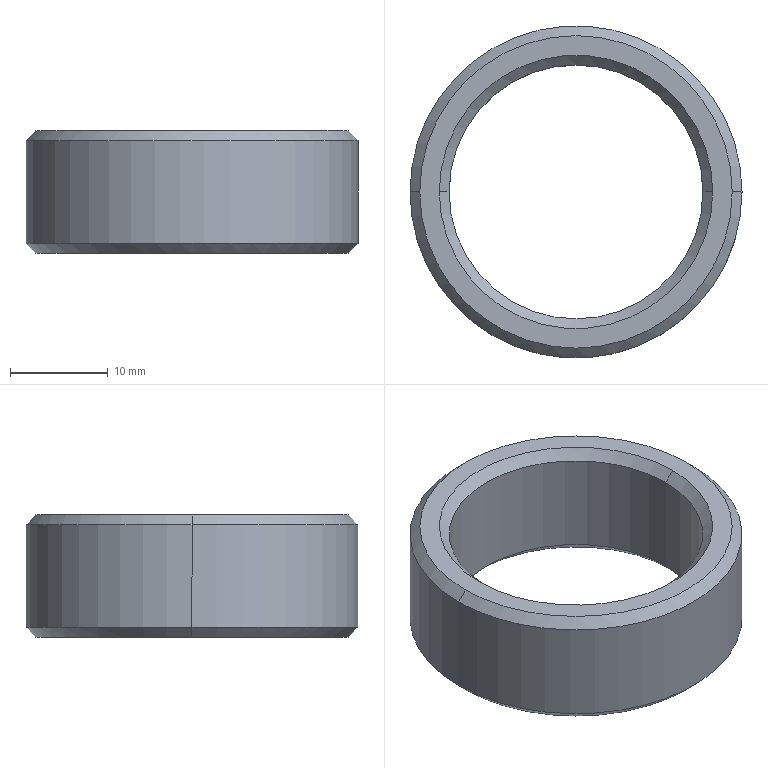Part | STEP file | 1 solid | 14 faces | box 34 x 34 x 12.5 mm | volume 4524 mm3 | cone 8 | cylinder 4 | plane 2 | commonest cylinder face diameters 26 x2 34 x2
STEP:
#1=CARTESIAN_POINT('',(0.,0.,0.));
#2=DIRECTION('',(0.,0.,1.));
#3=DIRECTION('',(1.,0.,0.));
#4=AXIS2_PLACEMENT_3D('',#1,#2,#3);
#5=CARTESIAN_POINT('',(-13.,0.,1.));
#6=VERTEX_POINT('',#5);
#7=CARTESIAN_POINT('',(13.,0.,1.));
#8=VERTEX_POINT('',#7);
#9=CARTESIAN_POINT('',(0.,0.,1.));
#10=DIRECTION('',(0.,0.,-1.));
#11=DIRECTION('',(-1.,0.,0.));
#12=AXIS2_PLACEMENT_3D('',#9,#10,#11);
#13=CIRCLE('',#12,13.);
#14=CARTESIAN_POINT('',(0.,0.,12.5));
#15=DIRECTION('',(0.,0.,-1.));
#16=DIRECTION('',(-1.,0.,0.));
#17=AXIS2_PLACEMENT_3D('',#14,#15,#16);
#18=CYLINDRICAL_SURFACE('',#17,13.);
#19=CARTESIAN_POINT('',(0.,11.5));
#20=DIRECTION('',(1.,0.));
#21=VECTOR('',#20,1.);
#22=LINE('',#19,#21);
#23=(GEOMETRIC_REPRESENTATION_CONTEXT(2)PARAMETRIC_REPRESENTATION_CONTEXT()REPRESENTATION_CONTEXT('',''));
#24=DEFINITIONAL_REPRESENTATION('',(#22),#23);
#25=PCURVE('',#18,#24);
#26=CARTESIAN_POINT('',(0.,0.,0.));
#27=DIRECTION('',(0.,0.,-1.));
#28=DIRECTION('',(-1.,0.,0.));
#29=AXIS2_PLACEMENT_3D('',#26,#27,#28);
#30=CONICAL_SURFACE('',#29,14.,0.7854);
#31=CARTESIAN_POINT('',(0.,-1.));
#32=DIRECTION('',(1.,0.));
#33=VECTOR('',#32,1.);
#34=LINE('',#31,#33);
#35=(GEOMETRIC_REPRESENTATION_CONTEXT(2)PARAMETRIC_REPRESENTATION_CONTEXT()REPRESENTATION_CONTEXT('',''));
#36=DEFINITIONAL_REPRESENTATION('',(#34),#35);
#37=PCURVE('',#30,#36);
#38=SURFACE_CURVE('',#13,(#25,#37),.PCURVE_S1.);
#39=EDGE_CURVE('',#6,#8,#38,.T.);
#40=ORIENTED_EDGE('',*,*,#39,.F.);
#41=CARTESIAN_POINT('',(-13.,0.,11.5));
#42=VERTEX_POINT('',#41);
#43=CARTESIAN_POINT('',(-13.,0.,12.5));
#44=DIRECTION('',(0.,0.,-1.));
#45=VECTOR('',#44,1.);
#46=LINE('',#43,#45);
#47=CARTESIAN_POINT('',(0.,0.));
#48=DIRECTION('',(0.,1.));
#49=VECTOR('',#48,1.);
#50=LINE('',#47,#49);
#51=(GEOMETRIC_REPRESENTATION_CONTEXT(2)PARAMETRIC_REPRESENTATION_CONTEXT()REPRESENTATION_CONTEXT('',''));
#52=DEFINITIONAL_REPRESENTATION('',(#50),#51);
#53=PCURVE('',#18,#52);
#54=CARTESIAN_POINT('',(0.,0.,12.5));
#55=DIRECTION('',(0.,0.,-1.));
#56=DIRECTION('',(-1.,0.,0.));
#57=AXIS2_PLACEMENT_3D('',#54,#55,#56);
#58=CYLINDRICAL_SURFACE('',#57,13.);
#59=CARTESIAN_POINT('',(6.283,0.));
#60=DIRECTION('',(0.,1.));
#61=VECTOR('',#60,1.);
#62=LINE('',#59,#61);
#63=(GEOMETRIC_REPRESENTATION_CONTEXT(2)PARAMETRIC_REPRESENTATION_CONTEXT()REPRESENTATION_CONTEXT('',''));
#64=DEFINITIONAL_REPRESENTATION('',(#62),#63);
#65=PCURVE('',#58,#64);
#66=SURFACE_CURVE('',#46,(#53,#65),.PCURVE_S1.);
#67=EDGE_CURVE('',#42,#6,#66,.T.);
#68=ORIENTED_EDGE('',*,*,#67,.F.);
#69=CARTESIAN_POINT('',(13.,0.,11.5));
#70=VERTEX_POINT('',#69);
#71=CARTESIAN_POINT('',(0.,0.,11.5));
#72=DIRECTION('',(0.,0.,1.));
#73=DIRECTION('',(1.,0.,0.));
#74=AXIS2_PLACEMENT_3D('',#71,#72,#73);
#75=CIRCLE('',#74,13.);
#76=CARTESIAN_POINT('',(3.142,1.));
#77=DIRECTION('',(-1.,0.));
#78=VECTOR('',#77,1.);
#79=LINE('',#76,#78);
#80=(GEOMETRIC_REPRESENTATION_CONTEXT(2)PARAMETRIC_REPRESENTATION_CONTEXT()REPRESENTATION_CONTEXT('',''));
#81=DEFINITIONAL_REPRESENTATION('',(#79),#80);
#82=PCURVE('',#18,#81);
#83=CARTESIAN_POINT('',(0.,0.,12.5));
#84=DIRECTION('',(0.,0.,1.));
#85=DIRECTION('',(1.,0.,0.));
#86=AXIS2_PLACEMENT_3D('',#83,#84,#85);
#87=CONICAL_SURFACE('',#86,14.,0.7854);
#88=CARTESIAN_POINT('',(0.,-1.));
#89=DIRECTION('',(1.,0.));
#90=VECTOR('',#89,1.);
#91=LINE('',#88,#90);
#92=(GEOMETRIC_REPRESENTATION_CONTEXT(2)PARAMETRIC_REPRESENTATION_CONTEXT()REPRESENTATION_CONTEXT('',''));
#93=DEFINITIONAL_REPRESENTATION('',(#91),#92);
#94=PCURVE('',#87,#93);
#95=SURFACE_CURVE('',#75,(#82,#94),.PCURVE_S1.);
#96=EDGE_CURVE('',#70,#42,#95,.T.);
#97=ORIENTED_EDGE('',*,*,#96,.F.);
#98=CARTESIAN_POINT('',(13.,0.,12.5));
#99=DIRECTION('',(0.,0.,-1.));
#100=VECTOR('',#99,1.);
#101=LINE('',#98,#100);
#102=CARTESIAN_POINT('',(3.142,0.));
#103=DIRECTION('',(0.,1.));
#104=VECTOR('',#103,1.);
#105=LINE('',#102,#104);
#106=(GEOMETRIC_REPRESENTATION_CONTEXT(2)PARAMETRIC_REPRESENTATION_CONTEXT()REPRESENTATION_CONTEXT('',''));
#107=DEFINITIONAL_REPRESENTATION('',(#105),#106);
#108=PCURVE('',#18,#107);
#109=CARTESIAN_POINT('',(3.142,0.));
#110=DIRECTION('',(0.,1.));
#111=VECTOR('',#110,1.);
#112=LINE('',#109,#111);
#113=(GEOMETRIC_REPRESENTATION_CONTEXT(2)PARAMETRIC_REPRESENTATION_CONTEXT()REPRESENTATION_CONTEXT('',''));
#114=DEFINITIONAL_REPRESENTATION('',(#112),#113);
#115=PCURVE('',#58,#114);
#116=SURFACE_CURVE('',#101,(#108,#115),.PCURVE_S1.);
#117=EDGE_CURVE('',#70,#8,#116,.T.);
#118=ORIENTED_EDGE('',*,*,#117,.T.);
#119=EDGE_LOOP('',(#40,#68,#97,#118));
#120=FACE_BOUND('',#119,.F.);
#121=ADVANCED_FACE('',(#120),#18,.F.);
#122=CARTESIAN_POINT('',(-14.,0.,12.5));
#123=VERTEX_POINT('',#122);
#124=CARTESIAN_POINT('',(14.,0.,12.5));
#125=VERTEX_POINT('',#124);
#126=CARTESIAN_POINT('',(0.,0.,12.5));
#127=DIRECTION('',(0.,0.,-1.));
#128=DIRECTION('',(1.,0.,0.));
#129=AXIS2_PLACEMENT_3D('',#126,#127,#128);
#130=CIRCLE('',#129,14.);
#131=CARTESIAN_POINT('',(6.283,0.));
#132=DIRECTION('',(-1.,0.));
#133=VECTOR('',#132,1.);
#134=LINE('',#131,#133);
#135=(GEOMETRIC_REPRESENTATION_CONTEXT(2)PARAMETRIC_REPRESENTATION_CONTEXT()REPRESENTATION_CONTEXT('',''));
#136=DEFINITIONAL_REPRESENTATION('',(#134),#135);
#137=PCURVE('',#87,#136);
#138=CARTESIAN_POINT('',(0.,0.,12.5));
#139=DIRECTION('',(0.,0.,1.));
#140=DIRECTION('',(1.,0.,0.));
#141=AXIS2_PLACEMENT_3D('',#138,#139,#140);
#142=PLANE('',#141);
#143=CARTESIAN_POINT('',(14.,0.));
#144=CARTESIAN_POINT('',(14.,-24.249));
#145=CARTESIAN_POINT('',(-7.,-12.124));
#146=CARTESIAN_POINT('',(-28.,0.));
#147=CARTESIAN_POINT('',(-7.,12.124));
#148=CARTESIAN_POINT('',(14.,24.249));
#149=CARTESIAN_POINT('',(14.,0.));
#150=(BOUNDED_CURVE()B_SPLINE_CURVE(2,(#143,#144,#145,#146,#147,#148,#149),.UNSPECIFIED.,.T.,.F.)B_SPLINE_CURVE_WITH_KNOTS((1,2,2,2,2,1),(-2.094,0.,2.094,4.189,6.283,8.378),.UNSPECIFIED.)CURVE()GEOMETRIC_REPRESENTATION_ITEM()RATIONAL_B_SPLINE_CURVE((1.,0.5,1.,0.5,1.,0.5,1.))REPRESENTATION_ITEM(''));
#151=(GEOMETRIC_REPRESENTATION_CONTEXT(2)PARAMETRIC_REPRESENTATION_CONTEXT()REPRESENTATION_CONTEXT('',''));
#152=DEFINITIONAL_REPRESENTATION('',(#150),#151);
#153=PCURVE('',#142,#152);
#154=SURFACE_CURVE('',#130,(#137,#153),.PCURVE_S1.);
#155=EDGE_CURVE('',#123,#125,#154,.T.);
#156=ORIENTED_EDGE('',*,*,#155,.T.);
#157=CARTESIAN_POINT('',(14.,0.,12.5));
#158=DIRECTION('',(0.7071,0.,0.7071));
#159=VECTOR('',#158,1.);
#160=LINE('',#157,#159);
#161=CARTESIAN_POINT('',(0.,0.));
#162=DIRECTION('',(0.,1.));
#163=VECTOR('',#162,1.);
#164=LINE('',#161,#163);
#165=(GEOMETRIC_REPRESENTATION_CONTEXT(2)PARAMETRIC_REPRESENTATION_CONTEXT()REPRESENTATION_CONTEXT('',''));
#166=DEFINITIONAL_REPRESENTATION('',(#164),#165);
#167=PCURVE('',#87,#166);
#168=CARTESIAN_POINT('',(0.,0.,12.5));
#169=DIRECTION('',(0.,0.,1.));
#170=DIRECTION('',(1.,0.,0.));
#171=AXIS2_PLACEMENT_3D('',#168,#169,#170);
#172=CONICAL_SURFACE('',#171,14.,0.7854);
#173=CARTESIAN_POINT('',(6.283,0.));
#174=DIRECTION('',(0.,1.));
#175=VECTOR('',#174,1.);
#176=LINE('',#173,#175);
#177=(GEOMETRIC_REPRESENTATION_CONTEXT(2)PARAMETRIC_REPRESENTATION_CONTEXT()REPRESENTATION_CONTEXT('',''));
#178=DEFINITIONAL_REPRESENTATION('',(#176),#177);
#179=PCURVE('',#172,#178);
#180=SURFACE_CURVE('',#160,(#167,#179),.PCURVE_S1.);
#181=EDGE_CURVE('',#70,#125,#180,.T.);
#182=ORIENTED_EDGE('',*,*,#181,.F.);
#183=ORIENTED_EDGE('',*,*,#96,.T.);
#184=CARTESIAN_POINT('',(-14.,0.,12.5));
#185=DIRECTION('',(-0.7071,0.,0.7071));
#186=VECTOR('',#185,1.);
#187=LINE('',#184,#186);
#188=CARTESIAN_POINT('',(3.142,0.));
#189=DIRECTION('',(0.,1.));
#190=VECTOR('',#189,1.);
#191=LINE('',#188,#190);
#192=(GEOMETRIC_REPRESENTATION_CONTEXT(2)PARAMETRIC_REPRESENTATION_CONTEXT()REPRESENTATION_CONTEXT('',''));
#193=DEFINITIONAL_REPRESENTATION('',(#191),#192);
#194=PCURVE('',#87,#193);
#195=CARTESIAN_POINT('',(3.142,0.));
#196=DIRECTION('',(0.,1.));
#197=VECTOR('',#196,1.);
#198=LINE('',#195,#197);
#199=(GEOMETRIC_REPRESENTATION_CONTEXT(2)PARAMETRIC_REPRESENTATION_CONTEXT()REPRESENTATION_CONTEXT('',''));
#200=DEFINITIONAL_REPRESENTATION('',(#198),#199);
#201=PCURVE('',#172,#200);
#202=SURFACE_CURVE('',#187,(#194,#201),.PCURVE_S1.);
#203=EDGE_CURVE('',#42,#123,#202,.T.);
#204=ORIENTED_EDGE('',*,*,#203,.T.);
#205=EDGE_LOOP('',(#156,#182,#183,#204));
#206=FACE_BOUND('',#205,.F.);
#207=ADVANCED_FACE('',(#206),#87,.F.);
#208=CARTESIAN_POINT('',(-14.,0.,0.));
#209=VERTEX_POINT('',#208);
#210=CARTESIAN_POINT('',(14.,0.,0.));
#211=VERTEX_POINT('',#210);
#212=CARTESIAN_POINT('',(0.,0.,0.));
#213=DIRECTION('',(0.,0.,-1.));
#214=DIRECTION('',(-1.,0.,0.));
#215=AXIS2_PLACEMENT_3D('',#212,#213,#214);
#216=CIRCLE('',#215,14.);
#217=CARTESIAN_POINT('',(0.,0.));
#218=DIRECTION('',(1.,0.));
#219=VECTOR('',#218,1.);
#220=LINE('',#217,#219);
#221=(GEOMETRIC_REPRESENTATION_CONTEXT(2)PARAMETRIC_REPRESENTATION_CONTEXT()REPRESENTATION_CONTEXT('',''));
#222=DEFINITIONAL_REPRESENTATION('',(#220),#221);
#223=PCURVE('',#30,#222);
#224=CARTESIAN_POINT('',(0.,0.,0.));
#225=DIRECTION('',(0.,0.,1.));
#226=DIRECTION('',(1.,0.,0.));
#227=AXIS2_PLACEMENT_3D('',#224,#225,#226);
#228=PLANE('',#227);
#229=CARTESIAN_POINT('',(-14.,0.));
#230=CARTESIAN_POINT('',(-14.,24.249));
#231=CARTESIAN_POINT('',(7.,12.124));
#232=CARTESIAN_POINT('',(28.,0.));
#233=CARTESIAN_POINT('',(7.,-12.124));
#234=CARTESIAN_POINT('',(-14.,-24.249));
#235=CARTESIAN_POINT('',(-14.,0.));
#236=(BOUNDED_CURVE()B_SPLINE_CURVE(2,(#229,#230,#231,#232,#233,#234,#235),.UNSPECIFIED.,.T.,.F.)B_SPLINE_CURVE_WITH_KNOTS((1,2,2,2,2,1),(-2.094,0.,2.094,4.189,6.283,8.378),.UNSPECIFIED.)CURVE()GEOMETRIC_REPRESENTATION_ITEM()RATIONAL_B_SPLINE_CURVE((1.,0.5,1.,0.5,1.,0.5,1.))REPRESENTATION_ITEM(''));
#237=(GEOMETRIC_REPRESENTATION_CONTEXT(2)PARAMETRIC_REPRESENTATION_CONTEXT()REPRESENTATION_CONTEXT('',''));
#238=DEFINITIONAL_REPRESENTATION('',(#236),#237);
#239=PCURVE('',#228,#238);
#240=SURFACE_CURVE('',#216,(#223,#239),.PCURVE_S1.);
#241=EDGE_CURVE('',#209,#211,#240,.T.);
#242=ORIENTED_EDGE('',*,*,#241,.F.);
#243=CARTESIAN_POINT('',(-14.,0.,0.));
#244=DIRECTION('',(-0.7071,0.,-0.7071));
#245=VECTOR('',#244,1.);
#246=LINE('',#243,#245);
#247=CARTESIAN_POINT('',(0.,0.));
#248=DIRECTION('',(0.,1.));
#249=VECTOR('',#248,1.);
#250=LINE('',#247,#249);
#251=(GEOMETRIC_REPRESENTATION_CONTEXT(2)PARAMETRIC_REPRESENTATION_CONTEXT()REPRESENTATION_CONTEXT('',''));
#252=DEFINITIONAL_REPRESENTATION('',(#250),#251);
#253=PCURVE('',#30,#252);
#254=CARTESIAN_POINT('',(0.,0.,0.));
#255=DIRECTION('',(0.,0.,-1.));
#256=DIRECTION('',(-1.,0.,0.));
#257=AXIS2_PLACEMENT_3D('',#254,#255,#256);
#258=CONICAL_SURFACE('',#257,14.,0.7854);
#259=CARTESIAN_POINT('',(6.283,0.));
#260=DIRECTION('',(0.,1.));
#261=VECTOR('',#260,1.);
#262=LINE('',#259,#261);
#263=(GEOMETRIC_REPRESENTATION_CONTEXT(2)PARAMETRIC_REPRESENTATION_CONTEXT()REPRESENTATION_CONTEXT('',''));
#264=DEFINITIONAL_REPRESENTATION('',(#262),#263);
#265=PCURVE('',#258,#264);
#266=SURFACE_CURVE('',#246,(#253,#265),.PCURVE_S1.);
#267=EDGE_CURVE('',#6,#209,#266,.T.);
#268=ORIENTED_EDGE('',*,*,#267,.F.);
#269=ORIENTED_EDGE('',*,*,#39,.T.);
#270=CARTESIAN_POINT('',(14.,0.,0.));
#271=DIRECTION('',(0.7071,0.,-0.7071));
#272=VECTOR('',#271,1.);
#273=LINE('',#270,#272);
#274=CARTESIAN_POINT('',(3.142,0.));
#275=DIRECTION('',(0.,1.));
#276=VECTOR('',#275,1.);
#277=LINE('',#274,#276);
#278=(GEOMETRIC_REPRESENTATION_CONTEXT(2)PARAMETRIC_REPRESENTATION_CONTEXT()REPRESENTATION_CONTEXT('',''));
#279=DEFINITIONAL_REPRESENTATION('',(#277),#278);
#280=PCURVE('',#30,#279);
#281=CARTESIAN_POINT('',(3.142,0.));
#282=DIRECTION('',(0.,1.));
#283=VECTOR('',#282,1.);
#284=LINE('',#281,#283);
#285=(GEOMETRIC_REPRESENTATION_CONTEXT(2)PARAMETRIC_REPRESENTATION_CONTEXT()REPRESENTATION_CONTEXT('',''));
#286=DEFINITIONAL_REPRESENTATION('',(#284),#285);
#287=PCURVE('',#258,#286);
#288=SURFACE_CURVE('',#273,(#280,#287),.PCURVE_S1.);
#289=EDGE_CURVE('',#8,#211,#288,.T.);
#290=ORIENTED_EDGE('',*,*,#289,.T.);
#291=EDGE_LOOP('',(#242,#268,#269,#290));
#292=FACE_BOUND('',#291,.F.);
#293=ADVANCED_FACE('',(#292),#30,.F.);
#294=CARTESIAN_POINT('',(0.,0.,12.5));
#295=DIRECTION('',(0.,0.,-1.));
#296=DIRECTION('',(1.,0.,0.));
#297=AXIS2_PLACEMENT_3D('',#294,#295,#296);
#298=CIRCLE('',#297,14.);
#299=CARTESIAN_POINT('',(14.,0.));
#300=CARTESIAN_POINT('',(14.,-24.249));
#301=CARTESIAN_POINT('',(-7.,-12.124));
#302=CARTESIAN_POINT('',(-28.,0.));
#303=CARTESIAN_POINT('',(-7.,12.124));
#304=CARTESIAN_POINT('',(14.,24.249));
#305=CARTESIAN_POINT('',(14.,0.));
#306=(BOUNDED_CURVE()B_SPLINE_CURVE(2,(#299,#300,#301,#302,#303,#304,#305),.UNSPECIFIED.,.T.,.F.)B_SPLINE_CURVE_WITH_KNOTS((1,2,2,2,2,1),(-2.094,0.,2.094,4.189,6.283,8.378),.UNSPECIFIED.)CURVE()GEOMETRIC_REPRESENTATION_ITEM()RATIONAL_B_SPLINE_CURVE((1.,0.5,1.,0.5,1.,0.5,1.))REPRESENTATION_ITEM(''));
#307=(GEOMETRIC_REPRESENTATION_CONTEXT(2)PARAMETRIC_REPRESENTATION_CONTEXT()REPRESENTATION_CONTEXT('',''));
#308=DEFINITIONAL_REPRESENTATION('',(#306),#307);
#309=PCURVE('',#142,#308);
#310=CARTESIAN_POINT('',(6.283,0.));
#311=DIRECTION('',(-1.,0.));
#312=VECTOR('',#311,1.);
#313=LINE('',#310,#312);
#314=(GEOMETRIC_REPRESENTATION_CONTEXT(2)PARAMETRIC_REPRESENTATION_CONTEXT()REPRESENTATION_CONTEXT('',''));
#315=DEFINITIONAL_REPRESENTATION('',(#313),#314);
#316=PCURVE('',#172,#315);
#317=SURFACE_CURVE('',#298,(#309,#316),.PCURVE_S1.);
#318=EDGE_CURVE('',#125,#123,#317,.T.);
#319=ORIENTED_EDGE('',*,*,#318,.T.);
#320=ORIENTED_EDGE('',*,*,#155,.T.);
#321=EDGE_LOOP('',(#319,#320));
#322=FACE_BOUND('',#321,.T.);
#323=CARTESIAN_POINT('',(-16.,0.,12.5));
#324=VERTEX_POINT('',#323);
#325=CARTESIAN_POINT('',(16.,0.,12.5));
#326=VERTEX_POINT('',#325);
#327=CARTESIAN_POINT('',(0.,0.,12.5));
#328=DIRECTION('',(0.,0.,-1.));
#329=DIRECTION('',(-1.,0.,0.));
#330=AXIS2_PLACEMENT_3D('',#327,#328,#329);
#331=CIRCLE('',#330,16.);
#332=CARTESIAN_POINT('',(-16.,0.));
#333=CARTESIAN_POINT('',(-16.,27.713));
#334=CARTESIAN_POINT('',(8.,13.856));
#335=CARTESIAN_POINT('',(32.,0.));
#336=CARTESIAN_POINT('',(8.,-13.856));
#337=CARTESIAN_POINT('',(-16.,-27.713));
#338=CARTESIAN_POINT('',(-16.,0.));
#339=(BOUNDED_CURVE()B_SPLINE_CURVE(2,(#332,#333,#334,#335,#336,#337,#338),.UNSPECIFIED.,.T.,.F.)B_SPLINE_CURVE_WITH_KNOTS((1,2,2,2,2,1),(-2.094,0.,2.094,4.189,6.283,8.378),.UNSPECIFIED.)CURVE()GEOMETRIC_REPRESENTATION_ITEM()RATIONAL_B_SPLINE_CURVE((1.,0.5,1.,0.5,1.,0.5,1.))REPRESENTATION_ITEM(''));
#340=(GEOMETRIC_REPRESENTATION_CONTEXT(2)PARAMETRIC_REPRESENTATION_CONTEXT()REPRESENTATION_CONTEXT('',''));
#341=DEFINITIONAL_REPRESENTATION('',(#339),#340);
#342=PCURVE('',#142,#341);
#343=CARTESIAN_POINT('',(0.,0.,11.5));
#344=DIRECTION('',(0.,0.,-1.));
#345=DIRECTION('',(-1.,0.,0.));
#346=AXIS2_PLACEMENT_3D('',#343,#344,#345);
#347=CONICAL_SURFACE('',#346,17.,0.7854);
#348=CARTESIAN_POINT('',(0.,-1.));
#349=DIRECTION('',(1.,0.));
#350=VECTOR('',#349,1.);
#351=LINE('',#348,#350);
#352=(GEOMETRIC_REPRESENTATION_CONTEXT(2)PARAMETRIC_REPRESENTATION_CONTEXT()REPRESENTATION_CONTEXT('',''));
#353=DEFINITIONAL_REPRESENTATION('',(#351),#352);
#354=PCURVE('',#347,#353);
#355=SURFACE_CURVE('',#331,(#342,#354),.PCURVE_S1.);
#356=EDGE_CURVE('',#324,#326,#355,.T.);
#357=ORIENTED_EDGE('',*,*,#356,.F.);
#358=CARTESIAN_POINT('',(0.,0.,12.5));
#359=DIRECTION('',(0.,0.,-1.));
#360=DIRECTION('',(-1.,0.,0.));
#361=AXIS2_PLACEMENT_3D('',#358,#359,#360);
#362=CIRCLE('',#361,16.);
#363=CARTESIAN_POINT('',(-16.,0.));
#364=CARTESIAN_POINT('',(-16.,27.713));
#365=CARTESIAN_POINT('',(8.,13.856));
#366=CARTESIAN_POINT('',(32.,0.));
#367=CARTESIAN_POINT('',(8.,-13.856));
#368=CARTESIAN_POINT('',(-16.,-27.713));
#369=CARTESIAN_POINT('',(-16.,0.));
#370=(BOUNDED_CURVE()B_SPLINE_CURVE(2,(#363,#364,#365,#366,#367,#368,#369),.UNSPECIFIED.,.T.,.F.)B_SPLINE_CURVE_WITH_KNOTS((1,2,2,2,2,1),(-2.094,0.,2.094,4.189,6.283,8.378),.UNSPECIFIED.)CURVE()GEOMETRIC_REPRESENTATION_ITEM()RATIONAL_B_SPLINE_CURVE((1.,0.5,1.,0.5,1.,0.5,1.))REPRESENTATION_ITEM(''));
#371=(GEOMETRIC_REPRESENTATION_CONTEXT(2)PARAMETRIC_REPRESENTATION_CONTEXT()REPRESENTATION_CONTEXT('',''));
#372=DEFINITIONAL_REPRESENTATION('',(#370),#371);
#373=PCURVE('',#142,#372);
#374=CARTESIAN_POINT('',(0.,0.,11.5));
#375=DIRECTION('',(0.,0.,-1.));
#376=DIRECTION('',(-1.,0.,0.));
#377=AXIS2_PLACEMENT_3D('',#374,#375,#376);
#378=CONICAL_SURFACE('',#377,17.,0.7854);
#379=CARTESIAN_POINT('',(0.,-1.));
#380=DIRECTION('',(1.,0.));
#381=VECTOR('',#380,1.);
#382=LINE('',#379,#381);
#383=(GEOMETRIC_REPRESENTATION_CONTEXT(2)PARAMETRIC_REPRESENTATION_CONTEXT()REPRESENTATION_CONTEXT('',''));
#384=DEFINITIONAL_REPRESENTATION('',(#382),#383);
#385=PCURVE('',#378,#384);
#386=SURFACE_CURVE('',#362,(#373,#385),.PCURVE_S1.);
#387=EDGE_CURVE('',#326,#324,#386,.T.);
#388=ORIENTED_EDGE('',*,*,#387,.F.);
#389=EDGE_LOOP('',(#357,#388));
#390=FACE_BOUND('',#389,.T.);
#391=ADVANCED_FACE('',(#322,#390),#142,.T.);
#392=ORIENTED_EDGE('',*,*,#241,.F.);
#393=CARTESIAN_POINT('',(0.,0.,0.));
#394=DIRECTION('',(0.,0.,-1.));
#395=DIRECTION('',(-1.,0.,0.));
#396=AXIS2_PLACEMENT_3D('',#393,#394,#395);
#397=CIRCLE('',#396,14.);
#398=CARTESIAN_POINT('',(-14.,0.));
#399=CARTESIAN_POINT('',(-14.,24.249));
#400=CARTESIAN_POINT('',(7.,12.124));
#401=CARTESIAN_POINT('',(28.,0.));
#402=CARTESIAN_POINT('',(7.,-12.124));
#403=CARTESIAN_POINT('',(-14.,-24.249));
#404=CARTESIAN_POINT('',(-14.,0.));
#405=(BOUNDED_CURVE()B_SPLINE_CURVE(2,(#398,#399,#400,#401,#402,#403,#404),.UNSPECIFIED.,.T.,.F.)B_SPLINE_CURVE_WITH_KNOTS((1,2,2,2,2,1),(-2.094,0.,2.094,4.189,6.283,8.378),.UNSPECIFIED.)CURVE()GEOMETRIC_REPRESENTATION_ITEM()RATIONAL_B_SPLINE_CURVE((1.,0.5,1.,0.5,1.,0.5,1.))REPRESENTATION_ITEM(''));
#406=(GEOMETRIC_REPRESENTATION_CONTEXT(2)PARAMETRIC_REPRESENTATION_CONTEXT()REPRESENTATION_CONTEXT('',''));
#407=DEFINITIONAL_REPRESENTATION('',(#405),#406);
#408=PCURVE('',#228,#407);
#409=CARTESIAN_POINT('',(0.,0.));
#410=DIRECTION('',(1.,0.));
#411=VECTOR('',#410,1.);
#412=LINE('',#409,#411);
#413=(GEOMETRIC_REPRESENTATION_CONTEXT(2)PARAMETRIC_REPRESENTATION_CONTEXT()REPRESENTATION_CONTEXT('',''));
#414=DEFINITIONAL_REPRESENTATION('',(#412),#413);
#415=PCURVE('',#258,#414);
#416=SURFACE_CURVE('',#397,(#408,#415),.PCURVE_S1.);
#417=EDGE_CURVE('',#211,#209,#416,.T.);
#418=ORIENTED_EDGE('',*,*,#417,.F.);
#419=EDGE_LOOP('',(#392,#418));
#420=FACE_BOUND('',#419,.T.);
#421=CARTESIAN_POINT('',(16.,0.,0.));
#422=VERTEX_POINT('',#421);
#423=CARTESIAN_POINT('',(-16.,0.,0.));
#424=VERTEX_POINT('',#423);
#425=CARTESIAN_POINT('',(0.,0.,0.));
#426=DIRECTION('',(0.,0.,1.));
#427=DIRECTION('',(1.,0.,0.));
#428=AXIS2_PLACEMENT_3D('',#425,#426,#427);
#429=CIRCLE('',#428,16.);
#430=CARTESIAN_POINT('',(0.,0.));
#431=DIRECTION('',(1.,0.));
#432=AXIS2_PLACEMENT_2D('',#430,#431);
#433=CIRCLE('',#432,16.);
#434=(GEOMETRIC_REPRESENTATION_CONTEXT(2)PARAMETRIC_REPRESENTATION_CONTEXT()REPRESENTATION_CONTEXT('',''));
#435=DEFINITIONAL_REPRESENTATION('',(#433),#434);
#436=PCURVE('',#228,#435);
#437=CARTESIAN_POINT('',(0.,0.,1.));
#438=DIRECTION('',(0.,0.,1.));
#439=DIRECTION('',(1.,0.,0.));
#440=AXIS2_PLACEMENT_3D('',#437,#438,#439);
#441=CONICAL_SURFACE('',#440,17.,0.7854);
#442=CARTESIAN_POINT('',(0.,-1.));
#443=DIRECTION('',(1.,0.));
#444=VECTOR('',#443,1.);
#445=LINE('',#442,#444);
#446=(GEOMETRIC_REPRESENTATION_CONTEXT(2)PARAMETRIC_REPRESENTATION_CONTEXT()REPRESENTATION_CONTEXT('',''));
#447=DEFINITIONAL_REPRESENTATION('',(#445),#446);
#448=PCURVE('',#441,#447);
#449=SURFACE_CURVE('',#429,(#436,#448),.PCURVE_S1.);
#450=EDGE_CURVE('',#422,#424,#449,.T.);
#451=ORIENTED_EDGE('',*,*,#450,.F.);
#452=CARTESIAN_POINT('',(0.,0.,0.));
#453=DIRECTION('',(0.,0.,1.));
#454=DIRECTION('',(1.,0.,0.));
#455=AXIS2_PLACEMENT_3D('',#452,#453,#454);
#456=CIRCLE('',#455,16.);
#457=CARTESIAN_POINT('',(0.,0.));
#458=DIRECTION('',(1.,0.));
#459=AXIS2_PLACEMENT_2D('',#457,#458);
#460=CIRCLE('',#459,16.);
#461=(GEOMETRIC_REPRESENTATION_CONTEXT(2)PARAMETRIC_REPRESENTATION_CONTEXT()REPRESENTATION_CONTEXT('',''));
#462=DEFINITIONAL_REPRESENTATION('',(#460),#461);
#463=PCURVE('',#228,#462);
#464=CARTESIAN_POINT('',(0.,0.,1.));
#465=DIRECTION('',(0.,0.,1.));
#466=DIRECTION('',(1.,0.,0.));
#467=AXIS2_PLACEMENT_3D('',#464,#465,#466);
#468=CONICAL_SURFACE('',#467,17.,0.7854);
#469=CARTESIAN_POINT('',(0.,-1.));
#470=DIRECTION('',(1.,0.));
#471=VECTOR('',#470,1.);
#472=LINE('',#469,#471);
#473=(GEOMETRIC_REPRESENTATION_CONTEXT(2)PARAMETRIC_REPRESENTATION_CONTEXT()REPRESENTATION_CONTEXT('',''));
#474=DEFINITIONAL_REPRESENTATION('',(#472),#473);
#475=PCURVE('',#468,#474);
#476=SURFACE_CURVE('',#456,(#463,#475),.PCURVE_S1.);
#477=EDGE_CURVE('',#424,#422,#476,.T.);
#478=ORIENTED_EDGE('',*,*,#477,.F.);
#479=EDGE_LOOP('',(#451,#478));
#480=FACE_BOUND('',#479,.T.);
#481=ADVANCED_FACE('',(#420,#480),#228,.F.);
#482=CARTESIAN_POINT('',(17.,0.,11.5));
#483=VERTEX_POINT('',#482);
#484=CARTESIAN_POINT('',(17.,0.,11.5));
#485=DIRECTION('',(0.7071,0.,-0.7071));
#486=VECTOR('',#485,1.);
#487=LINE('',#484,#486);
#488=CARTESIAN_POINT('',(3.142,0.));
#489=DIRECTION('',(0.,1.));
#490=VECTOR('',#489,1.);
#491=LINE('',#488,#490);
#492=(GEOMETRIC_REPRESENTATION_CONTEXT(2)PARAMETRIC_REPRESENTATION_CONTEXT()REPRESENTATION_CONTEXT('',''));
#493=DEFINITIONAL_REPRESENTATION('',(#491),#492);
#494=PCURVE('',#378,#493);
#495=CARTESIAN_POINT('',(3.142,0.));
#496=DIRECTION('',(0.,1.));
#497=VECTOR('',#496,1.);
#498=LINE('',#495,#497);
#499=(GEOMETRIC_REPRESENTATION_CONTEXT(2)PARAMETRIC_REPRESENTATION_CONTEXT()REPRESENTATION_CONTEXT('',''));
#500=DEFINITIONAL_REPRESENTATION('',(#498),#499);
#501=PCURVE('',#347,#500);
#502=SURFACE_CURVE('',#487,(#494,#501),.PCURVE_S1.);
#503=EDGE_CURVE('',#326,#483,#502,.T.);
#504=ORIENTED_EDGE('',*,*,#503,.F.);
#505=ORIENTED_EDGE('',*,*,#387,.T.);
#506=CARTESIAN_POINT('',(-17.,0.,11.5));
#507=VERTEX_POINT('',#506);
#508=CARTESIAN_POINT('',(-17.,0.,11.5));
#509=DIRECTION('',(-0.7071,0.,-0.7071));
#510=VECTOR('',#509,1.);
#511=LINE('',#508,#510);
#512=CARTESIAN_POINT('',(6.283,0.));
#513=DIRECTION('',(0.,1.));
#514=VECTOR('',#513,1.);
#515=LINE('',#512,#514);
#516=(GEOMETRIC_REPRESENTATION_CONTEXT(2)PARAMETRIC_REPRESENTATION_CONTEXT()REPRESENTATION_CONTEXT('',''));
#517=DEFINITIONAL_REPRESENTATION('',(#515),#516);
#518=PCURVE('',#378,#517);
#519=CARTESIAN_POINT('',(0.,0.));
#520=DIRECTION('',(0.,1.));
#521=VECTOR('',#520,1.);
#522=LINE('',#519,#521);
#523=(GEOMETRIC_REPRESENTATION_CONTEXT(2)PARAMETRIC_REPRESENTATION_CONTEXT()REPRESENTATION_CONTEXT('',''));
#524=DEFINITIONAL_REPRESENTATION('',(#522),#523);
#525=PCURVE('',#347,#524);
#526=SURFACE_CURVE('',#511,(#518,#525),.PCURVE_S1.);
#527=EDGE_CURVE('',#324,#507,#526,.T.);
#528=ORIENTED_EDGE('',*,*,#527,.T.);
#529=CARTESIAN_POINT('',(0.,0.,11.5));
#530=DIRECTION('',(0.,0.,-1.));
#531=DIRECTION('',(-1.,0.,0.));
#532=AXIS2_PLACEMENT_3D('',#529,#530,#531);
#533=CIRCLE('',#532,17.);
#534=CARTESIAN_POINT('',(0.,0.));
#535=DIRECTION('',(1.,0.));
#536=VECTOR('',#535,1.);
#537=LINE('',#534,#536);
#538=(GEOMETRIC_REPRESENTATION_CONTEXT(2)PARAMETRIC_REPRESENTATION_CONTEXT()REPRESENTATION_CONTEXT('',''));
#539=DEFINITIONAL_REPRESENTATION('',(#537),#538);
#540=PCURVE('',#378,#539);
#541=CARTESIAN_POINT('',(0.,0.,12.5));
#542=DIRECTION('',(0.,0.,-1.));
#543=DIRECTION('',(-1.,0.,0.));
#544=AXIS2_PLACEMENT_3D('',#541,#542,#543);
#545=CYLINDRICAL_SURFACE('',#544,17.);
#546=CARTESIAN_POINT('',(0.,1.));
#547=DIRECTION('',(1.,0.));
#548=VECTOR('',#547,1.);
#549=LINE('',#546,#548);
#550=(GEOMETRIC_REPRESENTATION_CONTEXT(2)PARAMETRIC_REPRESENTATION_CONTEXT()REPRESENTATION_CONTEXT('',''));
#551=DEFINITIONAL_REPRESENTATION('',(#549),#550);
#552=PCURVE('',#545,#551);
#553=SURFACE_CURVE('',#533,(#540,#552),.PCURVE_S1.);
#554=EDGE_CURVE('',#483,#507,#553,.T.);
#555=ORIENTED_EDGE('',*,*,#554,.F.);
#556=EDGE_LOOP('',(#504,#505,#528,#555));
#557=FACE_BOUND('',#556,.T.);
#558=ADVANCED_FACE('',(#557),#378,.T.);
#559=CARTESIAN_POINT('',(-17.,0.,1.));
#560=VERTEX_POINT('',#559);
#561=CARTESIAN_POINT('',(-17.,0.,1.));
#562=DIRECTION('',(-0.7071,0.,0.7071));
#563=VECTOR('',#562,1.);
#564=LINE('',#561,#563);
#565=CARTESIAN_POINT('',(3.142,0.));
#566=DIRECTION('',(0.,1.));
#567=VECTOR('',#566,1.);
#568=LINE('',#565,#567);
#569=(GEOMETRIC_REPRESENTATION_CONTEXT(2)PARAMETRIC_REPRESENTATION_CONTEXT()REPRESENTATION_CONTEXT('',''));
#570=DEFINITIONAL_REPRESENTATION('',(#568),#569);
#571=PCURVE('',#468,#570);
#572=CARTESIAN_POINT('',(3.142,0.));
#573=DIRECTION('',(0.,1.));
#574=VECTOR('',#573,1.);
#575=LINE('',#572,#574);
#576=(GEOMETRIC_REPRESENTATION_CONTEXT(2)PARAMETRIC_REPRESENTATION_CONTEXT()REPRESENTATION_CONTEXT('',''));
#577=DEFINITIONAL_REPRESENTATION('',(#575),#576);
#578=PCURVE('',#441,#577);
#579=SURFACE_CURVE('',#564,(#571,#578),.PCURVE_S1.);
#580=EDGE_CURVE('',#424,#560,#579,.T.);
#581=ORIENTED_EDGE('',*,*,#580,.F.);
#582=ORIENTED_EDGE('',*,*,#477,.T.);
#583=CARTESIAN_POINT('',(17.,0.,1.));
#584=VERTEX_POINT('',#583);
#585=CARTESIAN_POINT('',(17.,0.,1.));
#586=DIRECTION('',(0.7071,0.,0.7071));
#587=VECTOR('',#586,1.);
#588=LINE('',#585,#587);
#589=CARTESIAN_POINT('',(6.283,0.));
#590=DIRECTION('',(0.,1.));
#591=VECTOR('',#590,1.);
#592=LINE('',#589,#591);
#593=(GEOMETRIC_REPRESENTATION_CONTEXT(2)PARAMETRIC_REPRESENTATION_CONTEXT()REPRESENTATION_CONTEXT('',''));
#594=DEFINITIONAL_REPRESENTATION('',(#592),#593);
#595=PCURVE('',#468,#594);
#596=CARTESIAN_POINT('',(0.,0.));
#597=DIRECTION('',(0.,1.));
#598=VECTOR('',#597,1.);
#599=LINE('',#596,#598);
#600=(GEOMETRIC_REPRESENTATION_CONTEXT(2)PARAMETRIC_REPRESENTATION_CONTEXT()REPRESENTATION_CONTEXT('',''));
#601=DEFINITIONAL_REPRESENTATION('',(#599),#600);
#602=PCURVE('',#441,#601);
#603=SURFACE_CURVE('',#588,(#595,#602),.PCURVE_S1.);
#604=EDGE_CURVE('',#422,#584,#603,.T.);
#605=ORIENTED_EDGE('',*,*,#604,.T.);
#606=CARTESIAN_POINT('',(0.,0.,1.));
#607=DIRECTION('',(0.,0.,1.));
#608=DIRECTION('',(-1.,0.,0.));
#609=AXIS2_PLACEMENT_3D('',#606,#607,#608);
#610=CIRCLE('',#609,17.);
#611=CARTESIAN_POINT('',(3.142,0.));
#612=DIRECTION('',(1.,0.));
#613=VECTOR('',#612,1.);
#614=LINE('',#611,#613);
#615=(GEOMETRIC_REPRESENTATION_CONTEXT(2)PARAMETRIC_REPRESENTATION_CONTEXT()REPRESENTATION_CONTEXT('',''));
#616=DEFINITIONAL_REPRESENTATION('',(#614),#615);
#617=PCURVE('',#468,#616);
#618=CARTESIAN_POINT('',(6.283,11.5));
#619=DIRECTION('',(-1.,0.));
#620=VECTOR('',#619,1.);
#621=LINE('',#618,#620);
#622=(GEOMETRIC_REPRESENTATION_CONTEXT(2)PARAMETRIC_REPRESENTATION_CONTEXT()REPRESENTATION_CONTEXT('',''));
#623=DEFINITIONAL_REPRESENTATION('',(#621),#622);
#624=PCURVE('',#545,#623);
#625=SURFACE_CURVE('',#610,(#617,#624),.PCURVE_S1.);
#626=EDGE_CURVE('',#560,#584,#625,.T.);
#627=ORIENTED_EDGE('',*,*,#626,.F.);
#628=EDGE_LOOP('',(#581,#582,#605,#627));
#629=FACE_BOUND('',#628,.T.);
#630=ADVANCED_FACE('',(#629),#468,.T.);
#631=CARTESIAN_POINT('',(17.,0.,12.5));
#632=DIRECTION('',(0.,0.,-1.));
#633=VECTOR('',#632,1.);
#634=LINE('',#631,#633);
#635=CARTESIAN_POINT('',(3.142,0.));
#636=DIRECTION('',(0.,1.));
#637=VECTOR('',#636,1.);
#638=LINE('',#635,#637);
#639=(GEOMETRIC_REPRESENTATION_CONTEXT(2)PARAMETRIC_REPRESENTATION_CONTEXT()REPRESENTATION_CONTEXT('',''));
#640=DEFINITIONAL_REPRESENTATION('',(#638),#639);
#641=PCURVE('',#545,#640);
#642=CARTESIAN_POINT('',(0.,0.,12.5));
#643=DIRECTION('',(0.,0.,-1.));
#644=DIRECTION('',(-1.,0.,0.));
#645=AXIS2_PLACEMENT_3D('',#642,#643,#644);
#646=CYLINDRICAL_SURFACE('',#645,17.);
#647=CARTESIAN_POINT('',(3.142,0.));
#648=DIRECTION('',(0.,1.));
#649=VECTOR('',#648,1.);
#650=LINE('',#647,#649);
#651=(GEOMETRIC_REPRESENTATION_CONTEXT(2)PARAMETRIC_REPRESENTATION_CONTEXT()REPRESENTATION_CONTEXT('',''));
#652=DEFINITIONAL_REPRESENTATION('',(#650),#651);
#653=PCURVE('',#646,#652);
#654=SURFACE_CURVE('',#634,(#641,#653),.PCURVE_S1.);
#655=EDGE_CURVE('',#483,#584,#654,.T.);
#656=ORIENTED_EDGE('',*,*,#655,.F.);
#657=ORIENTED_EDGE('',*,*,#554,.T.);
#658=CARTESIAN_POINT('',(-17.,0.,12.5));
#659=DIRECTION('',(0.,0.,-1.));
#660=VECTOR('',#659,1.);
#661=LINE('',#658,#660);
#662=CARTESIAN_POINT('',(6.283,0.));
#663=DIRECTION('',(0.,1.));
#664=VECTOR('',#663,1.);
#665=LINE('',#662,#664);
#666=(GEOMETRIC_REPRESENTATION_CONTEXT(2)PARAMETRIC_REPRESENTATION_CONTEXT()REPRESENTATION_CONTEXT('',''));
#667=DEFINITIONAL_REPRESENTATION('',(#665),#666);
#668=PCURVE('',#545,#667);
#669=CARTESIAN_POINT('',(0.,0.));
#670=DIRECTION('',(0.,1.));
#671=VECTOR('',#670,1.);
#672=LINE('',#669,#671);
#673=(GEOMETRIC_REPRESENTATION_CONTEXT(2)PARAMETRIC_REPRESENTATION_CONTEXT()REPRESENTATION_CONTEXT('',''));
#674=DEFINITIONAL_REPRESENTATION('',(#672),#673);
#675=PCURVE('',#646,#674);
#676=SURFACE_CURVE('',#661,(#668,#675),.PCURVE_S1.);
#677=EDGE_CURVE('',#507,#560,#676,.T.);
#678=ORIENTED_EDGE('',*,*,#677,.T.);
#679=ORIENTED_EDGE('',*,*,#626,.T.);
#680=EDGE_LOOP('',(#656,#657,#678,#679));
#681=FACE_BOUND('',#680,.T.);
#682=ADVANCED_FACE('',(#681),#545,.T.);
#683=ORIENTED_EDGE('',*,*,#67,.T.);
#684=CARTESIAN_POINT('',(0.,0.,1.));
#685=DIRECTION('',(0.,0.,-1.));
#686=DIRECTION('',(-1.,0.,0.));
#687=AXIS2_PLACEMENT_3D('',#684,#685,#686);
#688=CIRCLE('',#687,13.);
#689=CARTESIAN_POINT('',(0.,11.5));
#690=DIRECTION('',(1.,0.));
#691=VECTOR('',#690,1.);
#692=LINE('',#689,#691);
#693=(GEOMETRIC_REPRESENTATION_CONTEXT(2)PARAMETRIC_REPRESENTATION_CONTEXT()REPRESENTATION_CONTEXT('',''));
#694=DEFINITIONAL_REPRESENTATION('',(#692),#693);
#695=PCURVE('',#58,#694);
#696=CARTESIAN_POINT('',(0.,-1.));
#697=DIRECTION('',(1.,0.));
#698=VECTOR('',#697,1.);
#699=LINE('',#696,#698);
#700=(GEOMETRIC_REPRESENTATION_CONTEXT(2)PARAMETRIC_REPRESENTATION_CONTEXT()REPRESENTATION_CONTEXT('',''));
#701=DEFINITIONAL_REPRESENTATION('',(#699),#700);
#702=PCURVE('',#258,#701);
#703=SURFACE_CURVE('',#688,(#695,#702),.PCURVE_S1.);
#704=EDGE_CURVE('',#8,#6,#703,.T.);
#705=ORIENTED_EDGE('',*,*,#704,.F.);
#706=ORIENTED_EDGE('',*,*,#117,.F.);
#707=CARTESIAN_POINT('',(0.,0.,11.5));
#708=DIRECTION('',(0.,0.,1.));
#709=DIRECTION('',(1.,0.,0.));
#710=AXIS2_PLACEMENT_3D('',#707,#708,#709);
#711=CIRCLE('',#710,13.);
#712=CARTESIAN_POINT('',(9.425,1.));
#713=DIRECTION('',(-1.,0.));
#714=VECTOR('',#713,1.);
#715=LINE('',#712,#714);
#716=(GEOMETRIC_REPRESENTATION_CONTEXT(2)PARAMETRIC_REPRESENTATION_CONTEXT()REPRESENTATION_CONTEXT('',''));
#717=DEFINITIONAL_REPRESENTATION('',(#715),#716);
#718=PCURVE('',#58,#717);
#719=CARTESIAN_POINT('',(0.,-1.));
#720=DIRECTION('',(1.,0.));
#721=VECTOR('',#720,1.);
#722=LINE('',#719,#721);
#723=(GEOMETRIC_REPRESENTATION_CONTEXT(2)PARAMETRIC_REPRESENTATION_CONTEXT()REPRESENTATION_CONTEXT('',''));
#724=DEFINITIONAL_REPRESENTATION('',(#722),#723);
#725=PCURVE('',#172,#724);
#726=SURFACE_CURVE('',#711,(#718,#725),.PCURVE_S1.);
#727=EDGE_CURVE('',#42,#70,#726,.T.);
#728=ORIENTED_EDGE('',*,*,#727,.F.);
#729=EDGE_LOOP('',(#683,#705,#706,#728));
#730=FACE_BOUND('',#729,.F.);
#731=ADVANCED_FACE('',(#730),#58,.F.);
#732=ORIENTED_EDGE('',*,*,#181,.T.);
#733=ORIENTED_EDGE('',*,*,#318,.T.);
#734=ORIENTED_EDGE('',*,*,#203,.F.);
#735=ORIENTED_EDGE('',*,*,#727,.T.);
#736=EDGE_LOOP('',(#732,#733,#734,#735));
#737=FACE_BOUND('',#736,.F.);
#738=ADVANCED_FACE('',(#737),#172,.F.);
#739=ORIENTED_EDGE('',*,*,#267,.T.);
#740=ORIENTED_EDGE('',*,*,#417,.F.);
#741=ORIENTED_EDGE('',*,*,#289,.F.);
#742=ORIENTED_EDGE('',*,*,#704,.T.);
#743=EDGE_LOOP('',(#739,#740,#741,#742));
#744=FACE_BOUND('',#743,.F.);
#745=ADVANCED_FACE('',(#744),#258,.F.);
#746=ORIENTED_EDGE('',*,*,#356,.T.);
#747=ORIENTED_EDGE('',*,*,#503,.T.);
#748=CARTESIAN_POINT('',(0.,0.,11.5));
#749=DIRECTION('',(0.,0.,-1.));
#750=DIRECTION('',(-1.,0.,0.));
#751=AXIS2_PLACEMENT_3D('',#748,#749,#750);
#752=CIRCLE('',#751,17.);
#753=CARTESIAN_POINT('',(0.,0.));
#754=DIRECTION('',(1.,0.));
#755=VECTOR('',#754,1.);
#756=LINE('',#753,#755);
#757=(GEOMETRIC_REPRESENTATION_CONTEXT(2)PARAMETRIC_REPRESENTATION_CONTEXT()REPRESENTATION_CONTEXT('',''));
#758=DEFINITIONAL_REPRESENTATION('',(#756),#757);
#759=PCURVE('',#347,#758);
#760=CARTESIAN_POINT('',(0.,1.));
#761=DIRECTION('',(1.,0.));
#762=VECTOR('',#761,1.);
#763=LINE('',#760,#762);
#764=(GEOMETRIC_REPRESENTATION_CONTEXT(2)PARAMETRIC_REPRESENTATION_CONTEXT()REPRESENTATION_CONTEXT('',''));
#765=DEFINITIONAL_REPRESENTATION('',(#763),#764);
#766=PCURVE('',#646,#765);
#767=SURFACE_CURVE('',#752,(#759,#766),.PCURVE_S1.);
#768=EDGE_CURVE('',#507,#483,#767,.T.);
#769=ORIENTED_EDGE('',*,*,#768,.F.);
#770=ORIENTED_EDGE('',*,*,#527,.F.);
#771=EDGE_LOOP('',(#746,#747,#769,#770));
#772=FACE_BOUND('',#771,.T.);
#773=ADVANCED_FACE('',(#772),#347,.T.);
#774=ORIENTED_EDGE('',*,*,#450,.T.);
#775=ORIENTED_EDGE('',*,*,#580,.T.);
#776=CARTESIAN_POINT('',(0.,0.,1.));
#777=DIRECTION('',(0.,0.,1.));
#778=DIRECTION('',(-1.,0.,0.));
#779=AXIS2_PLACEMENT_3D('',#776,#777,#778);
#780=CIRCLE('',#779,17.);
#781=CARTESIAN_POINT('',(-3.142,0.));
#782=DIRECTION('',(1.,0.));
#783=VECTOR('',#782,1.);
#784=LINE('',#781,#783);
#785=(GEOMETRIC_REPRESENTATION_CONTEXT(2)PARAMETRIC_REPRESENTATION_CONTEXT()REPRESENTATION_CONTEXT('',''));
#786=DEFINITIONAL_REPRESENTATION('',(#784),#785);
#787=PCURVE('',#441,#786);
#788=CARTESIAN_POINT('',(6.283,11.5));
#789=DIRECTION('',(-1.,0.));
#790=VECTOR('',#789,1.);
#791=LINE('',#788,#790);
#792=(GEOMETRIC_REPRESENTATION_CONTEXT(2)PARAMETRIC_REPRESENTATION_CONTEXT()REPRESENTATION_CONTEXT('',''));
#793=DEFINITIONAL_REPRESENTATION('',(#791),#792);
#794=PCURVE('',#646,#793);
#795=SURFACE_CURVE('',#780,(#787,#794),.PCURVE_S1.);
#796=EDGE_CURVE('',#584,#560,#795,.T.);
#797=ORIENTED_EDGE('',*,*,#796,.F.);
#798=ORIENTED_EDGE('',*,*,#604,.F.);
#799=EDGE_LOOP('',(#774,#775,#797,#798));
#800=FACE_BOUND('',#799,.T.);
#801=ADVANCED_FACE('',(#800),#441,.T.);
#802=ORIENTED_EDGE('',*,*,#768,.T.);
#803=ORIENTED_EDGE('',*,*,#655,.T.);
#804=ORIENTED_EDGE('',*,*,#796,.T.);
#805=ORIENTED_EDGE('',*,*,#677,.F.);
#806=EDGE_LOOP('',(#802,#803,#804,#805));
#807=FACE_BOUND('',#806,.T.);
#808=ADVANCED_FACE('',(#807),#646,.T.);
#809=CLOSED_SHELL('',(#121,#207,#293,#391,#481,#558,#630,#682,#731,#738,#745,#773,#801,#808));
#810=MANIFOLD_SOLID_BREP('',#809);
#811=(LENGTH_UNIT()NAMED_UNIT(*)SI_UNIT(.MILLI.,.METRE.));
#812=UNCERTAINTY_MEASURE_WITH_UNIT(LENGTH_MEASURE(0.0000001),#811,'','');
#813=(NAMED_UNIT(*)PLANE_ANGLE_UNIT()SI_UNIT($,.RADIAN.));
#814=(NAMED_UNIT(*)SI_UNIT($,.STERADIAN.)SOLID_ANGLE_UNIT());
#815=(GEOMETRIC_REPRESENTATION_CONTEXT(3)GLOBAL_UNCERTAINTY_ASSIGNED_CONTEXT((#812))GLOBAL_UNIT_ASSIGNED_CONTEXT((#811,#813,#814))REPRESENTATION_CONTEXT('',''));
#816=ADVANCED_BREP_SHAPE_REPRESENTATION('',(#4,#810),#815);